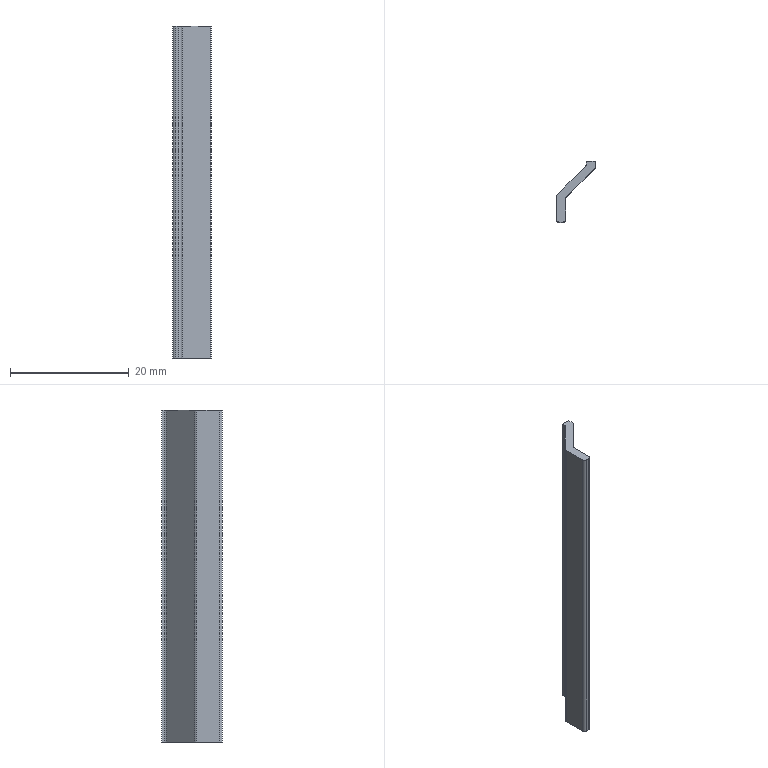Part | NX | features BREP 2 | 2 solids | 32 faces | box 6.515 x 10.276 x 56 mm | volume 1939 mm3 | plane 20 | cylinder 12 | commonest cylinder face diameters 1 x12
STEP:
#1=CARTESIAN_POINT('',(3.258,4.27,-4.));
#2=VERTEX_POINT('',#1);
#3=CARTESIAN_POINT('',(3.258,4.27,52.));
#4=VERTEX_POINT('',#3);
#5=CARTESIAN_POINT('',(3.258,4.27,0.));
#6=DIRECTION('',(0.,0.,1.));
#7=VECTOR('',#6,1000.);
#8=LINE('',#5,#7);
#9=EDGE_CURVE('',#2,#4,#8,.T.);
#10=ORIENTED_EDGE('',*,*,#9,.T.);
#11=CARTESIAN_POINT('',(3.111,3.917,52.));
#12=VERTEX_POINT('',#11);
#13=CARTESIAN_POINT('',(2.758,4.27,52.));
#14=DIRECTION('',(0.,0.,1.));
#15=DIRECTION('',(1.,0.,0.));
#16=AXIS2_PLACEMENT_3D('',#13,#14,#15);
#17=CIRCLE('',#16,0.5);
#18=EDGE_CURVE('',#12,#4,#17,.T.);
#19=ORIENTED_EDGE('',*,*,#18,.F.);
#20=CARTESIAN_POINT('',(3.111,3.917,-4.));
#21=VERTEX_POINT('',#20);
#22=CARTESIAN_POINT('',(3.111,3.917,0.));
#23=DIRECTION('',(0.,0.,1.));
#24=VECTOR('',#23,1000.);
#25=LINE('',#22,#24);
#26=EDGE_CURVE('',#21,#12,#25,.T.);
#27=ORIENTED_EDGE('',*,*,#26,.F.);
#28=CARTESIAN_POINT('',(2.758,4.27,-4.));
#29=DIRECTION('',(0.,0.,1.));
#30=DIRECTION('',(1.,0.,0.));
#31=AXIS2_PLACEMENT_3D('',#28,#29,#30);
#32=CIRCLE('',#31,0.5);
#33=EDGE_CURVE('',#21,#2,#32,.T.);
#34=ORIENTED_EDGE('',*,*,#33,.T.);
#35=EDGE_LOOP('',(#10,#19,#27,#34));
#36=FACE_BOUND('',#35,.T.);
#37=CARTESIAN_POINT('',(2.758,4.27,0.));
#38=DIRECTION('',(0.,0.,1.));
#39=DIRECTION('',(-1.,0.,0.));
#40=AXIS2_PLACEMENT_3D('',#37,#38,#39);
#41=CYLINDRICAL_SURFACE('',#40,0.5);
#42=ADVANCED_FACE('',(#36),#41,.T.);
#43=ORIENTED_EDGE('',*,*,#26,.T.);
#44=CARTESIAN_POINT('',(-1.611,-0.806,52.));
#45=VERTEX_POINT('',#44);
#46=CARTESIAN_POINT('',(3.111,3.917,52.));
#47=DIRECTION('',(0.7071,0.7071,0.));
#48=VECTOR('',#47,1000.);
#49=LINE('',#46,#48);
#50=EDGE_CURVE('',#45,#12,#49,.T.);
#51=ORIENTED_EDGE('',*,*,#50,.F.);
#52=CARTESIAN_POINT('',(-1.611,-0.806,-4.));
#53=VERTEX_POINT('',#52);
#54=CARTESIAN_POINT('',(-1.611,-0.806,0.));
#55=DIRECTION('',(0.,0.,1.));
#56=VECTOR('',#55,1000.);
#57=LINE('',#54,#56);
#58=EDGE_CURVE('',#53,#45,#57,.T.);
#59=ORIENTED_EDGE('',*,*,#58,.F.);
#60=CARTESIAN_POINT('',(3.111,3.917,-4.));
#61=DIRECTION('',(0.7071,0.7071,0.));
#62=VECTOR('',#61,1000.);
#63=LINE('',#60,#62);
#64=EDGE_CURVE('',#53,#21,#63,.T.);
#65=ORIENTED_EDGE('',*,*,#64,.T.);
#66=EDGE_LOOP('',(#43,#51,#59,#65));
#67=FACE_BOUND('',#66,.T.);
#68=CARTESIAN_POINT('',(3.111,3.917,0.));
#69=DIRECTION('',(-0.7071,0.7071,0.));
#70=DIRECTION('',(0.7071,0.7071,0.));
#71=AXIS2_PLACEMENT_3D('',#68,#69,#70);
#72=PLANE('',#71);
#73=ADVANCED_FACE('',(#67),#72,.F.);
#74=ORIENTED_EDGE('',*,*,#58,.T.);
#75=CARTESIAN_POINT('',(-1.758,-1.16,52.));
#76=VERTEX_POINT('',#75);
#77=CARTESIAN_POINT('',(-1.258,-1.16,52.));
#78=DIRECTION('',(0.,0.,-1.));
#79=DIRECTION('',(1.,0.,0.));
#80=AXIS2_PLACEMENT_3D('',#77,#78,#79);
#81=CIRCLE('',#80,0.5);
#82=EDGE_CURVE('',#76,#45,#81,.T.);
#83=ORIENTED_EDGE('',*,*,#82,.F.);
#84=CARTESIAN_POINT('',(-1.758,-1.16,-4.));
#85=VERTEX_POINT('',#84);
#86=CARTESIAN_POINT('',(-1.758,-1.16,0.));
#87=DIRECTION('',(0.,0.,1.));
#88=VECTOR('',#87,1000.);
#89=LINE('',#86,#88);
#90=EDGE_CURVE('',#85,#76,#89,.T.);
#91=ORIENTED_EDGE('',*,*,#90,.F.);
#92=CARTESIAN_POINT('',(-1.258,-1.16,-4.));
#93=DIRECTION('',(0.,0.,-1.));
#94=DIRECTION('',(1.,0.,0.));
#95=AXIS2_PLACEMENT_3D('',#92,#93,#94);
#96=CIRCLE('',#95,0.5);
#97=EDGE_CURVE('',#85,#53,#96,.T.);
#98=ORIENTED_EDGE('',*,*,#97,.T.);
#99=EDGE_LOOP('',(#74,#83,#91,#98));
#100=FACE_BOUND('',#99,.T.);
#101=CARTESIAN_POINT('',(-1.258,-1.16,0.));
#102=DIRECTION('',(0.,0.,1.));
#103=DIRECTION('',(-1.,0.,0.));
#104=AXIS2_PLACEMENT_3D('',#101,#102,#103);
#105=CYLINDRICAL_SURFACE('',#104,0.5);
#106=ADVANCED_FACE('',(#100),#105,.F.);
#107=ORIENTED_EDGE('',*,*,#90,.T.);
#108=CARTESIAN_POINT('',(-1.758,-4.613,52.));
#109=VERTEX_POINT('',#108);
#110=CARTESIAN_POINT('',(-1.758,-7.135,52.));
#111=DIRECTION('',(0.,1.,0.));
#112=VECTOR('',#111,1000.);
#113=LINE('',#110,#112);
#114=EDGE_CURVE('',#109,#76,#113,.T.);
#115=ORIENTED_EDGE('',*,*,#114,.F.);
#116=CARTESIAN_POINT('',(-1.758,-4.613,-4.));
#117=VERTEX_POINT('',#116);
#118=CARTESIAN_POINT('',(-1.758,-4.613,0.));
#119=DIRECTION('',(0.,0.,1.));
#120=VECTOR('',#119,1000.);
#121=LINE('',#118,#120);
#122=EDGE_CURVE('',#117,#109,#121,.T.);
#123=ORIENTED_EDGE('',*,*,#122,.F.);
#124=CARTESIAN_POINT('',(-1.758,-7.135,-4.));
#125=DIRECTION('',(0.,1.,0.));
#126=VECTOR('',#125,1000.);
#127=LINE('',#124,#126);
#128=EDGE_CURVE('',#117,#85,#127,.T.);
#129=ORIENTED_EDGE('',*,*,#128,.T.);
#130=EDGE_LOOP('',(#107,#115,#123,#129));
#131=FACE_BOUND('',#130,.T.);
#132=CARTESIAN_POINT('',(-1.758,-1.16,0.));
#133=DIRECTION('',(-1.,0.,0.));
#134=DIRECTION('',(0.,1.,0.));
#135=AXIS2_PLACEMENT_3D('',#132,#133,#134);
#136=PLANE('',#135);
#137=ADVANCED_FACE('',(#131),#136,.F.);
#138=ORIENTED_EDGE('',*,*,#122,.T.);
#139=CARTESIAN_POINT('',(-2.258,-5.113,52.));
#140=VERTEX_POINT('',#139);
#141=CARTESIAN_POINT('',(-2.258,-4.613,52.));
#142=DIRECTION('',(0.,0.,1.));
#143=DIRECTION('',(1.,0.,0.));
#144=AXIS2_PLACEMENT_3D('',#141,#142,#143);
#145=CIRCLE('',#144,0.5);
#146=EDGE_CURVE('',#140,#109,#145,.T.);
#147=ORIENTED_EDGE('',*,*,#146,.F.);
#148=CARTESIAN_POINT('',(-2.258,-5.113,-4.));
#149=VERTEX_POINT('',#148);
#150=CARTESIAN_POINT('',(-2.258,-5.113,0.));
#151=DIRECTION('',(0.,0.,1.));
#152=VECTOR('',#151,1000.);
#153=LINE('',#150,#152);
#154=EDGE_CURVE('',#149,#140,#153,.T.);
#155=ORIENTED_EDGE('',*,*,#154,.F.);
#156=CARTESIAN_POINT('',(-2.258,-4.613,-4.));
#157=DIRECTION('',(0.,0.,1.));
#158=DIRECTION('',(1.,0.,0.));
#159=AXIS2_PLACEMENT_3D('',#156,#157,#158);
#160=CIRCLE('',#159,0.5);
#161=EDGE_CURVE('',#149,#117,#160,.T.);
#162=ORIENTED_EDGE('',*,*,#161,.T.);
#163=EDGE_LOOP('',(#138,#147,#155,#162));
#164=FACE_BOUND('',#163,.T.);
#165=CARTESIAN_POINT('',(-2.258,-4.613,0.));
#166=DIRECTION('',(0.,0.,1.));
#167=DIRECTION('',(-1.,0.,0.));
#168=AXIS2_PLACEMENT_3D('',#165,#166,#167);
#169=CYLINDRICAL_SURFACE('',#168,0.5);
#170=ADVANCED_FACE('',(#164),#169,.T.);
#171=ORIENTED_EDGE('',*,*,#154,.T.);
#172=CARTESIAN_POINT('',(-2.758,-5.113,52.));
#173=VERTEX_POINT('',#172);
#174=CARTESIAN_POINT('',(2.716,-5.113,52.));
#175=DIRECTION('',(1.,0.,0.));
#176=VECTOR('',#175,1000.);
#177=LINE('',#174,#176);
#178=EDGE_CURVE('',#173,#140,#177,.T.);
#179=ORIENTED_EDGE('',*,*,#178,.F.);
#180=CARTESIAN_POINT('',(-2.758,-5.113,-4.));
#181=VERTEX_POINT('',#180);
#182=CARTESIAN_POINT('',(-2.758,-5.113,0.));
#183=DIRECTION('',(0.,0.,1.));
#184=VECTOR('',#183,1000.);
#185=LINE('',#182,#184);
#186=EDGE_CURVE('',#181,#173,#185,.T.);
#187=ORIENTED_EDGE('',*,*,#186,.F.);
#188=CARTESIAN_POINT('',(2.716,-5.113,-4.));
#189=DIRECTION('',(1.,0.,0.));
#190=VECTOR('',#189,1000.);
#191=LINE('',#188,#190);
#192=EDGE_CURVE('',#181,#149,#191,.T.);
#193=ORIENTED_EDGE('',*,*,#192,.T.);
#194=EDGE_LOOP('',(#171,#179,#187,#193));
#195=FACE_BOUND('',#194,.T.);
#196=CARTESIAN_POINT('',(-2.258,-5.113,0.));
#197=DIRECTION('',(0.,1.,0.));
#198=DIRECTION('',(1.,0.,0.));
#199=AXIS2_PLACEMENT_3D('',#196,#197,#198);
#200=PLANE('',#199);
#201=ADVANCED_FACE('',(#195),#200,.F.);
#202=ORIENTED_EDGE('',*,*,#186,.T.);
#203=CARTESIAN_POINT('',(-3.258,-4.613,52.));
#204=VERTEX_POINT('',#203);
#205=CARTESIAN_POINT('',(-2.758,-4.613,52.));
#206=DIRECTION('',(0.,0.,1.));
#207=DIRECTION('',(1.,0.,0.));
#208=AXIS2_PLACEMENT_3D('',#205,#206,#207);
#209=CIRCLE('',#208,0.5);
#210=EDGE_CURVE('',#204,#173,#209,.T.);
#211=ORIENTED_EDGE('',*,*,#210,.F.);
#212=CARTESIAN_POINT('',(-3.258,-4.613,-4.));
#213=VERTEX_POINT('',#212);
#214=CARTESIAN_POINT('',(-3.258,-4.613,0.));
#215=DIRECTION('',(0.,0.,1.));
#216=VECTOR('',#215,1000.);
#217=LINE('',#214,#216);
#218=EDGE_CURVE('',#213,#204,#217,.T.);
#219=ORIENTED_EDGE('',*,*,#218,.F.);
#220=CARTESIAN_POINT('',(-2.758,-4.613,-4.));
#221=DIRECTION('',(0.,0.,1.));
#222=DIRECTION('',(1.,0.,0.));
#223=AXIS2_PLACEMENT_3D('',#220,#221,#222);
#224=CIRCLE('',#223,0.5);
#225=EDGE_CURVE('',#213,#181,#224,.T.);
#226=ORIENTED_EDGE('',*,*,#225,.T.);
#227=EDGE_LOOP('',(#202,#211,#219,#226));
#228=FACE_BOUND('',#227,.T.);
#229=CARTESIAN_POINT('',(-2.758,-4.613,0.));
#230=DIRECTION('',(0.,0.,1.));
#231=DIRECTION('',(-1.,0.,0.));
#232=AXIS2_PLACEMENT_3D('',#229,#230,#231);
#233=CYLINDRICAL_SURFACE('',#232,0.5);
#234=ADVANCED_FACE('',(#228),#233,.T.);
#235=ORIENTED_EDGE('',*,*,#218,.T.);
#236=CARTESIAN_POINT('',(-3.258,-0.7595,52.));
#237=VERTEX_POINT('',#236);
#238=CARTESIAN_POINT('',(-3.258,-7.135,52.));
#239=DIRECTION('',(0.,-1.,0.));
#240=VECTOR('',#239,1000.);
#241=LINE('',#238,#240);
#242=EDGE_CURVE('',#237,#204,#241,.T.);
#243=ORIENTED_EDGE('',*,*,#242,.F.);
#244=CARTESIAN_POINT('',(-3.258,-0.7595,-4.));
#245=VERTEX_POINT('',#244);
#246=CARTESIAN_POINT('',(-3.258,-0.7595,0.));
#247=DIRECTION('',(0.,0.,1.));
#248=VECTOR('',#247,1000.);
#249=LINE('',#246,#248);
#250=EDGE_CURVE('',#245,#237,#249,.T.);
#251=ORIENTED_EDGE('',*,*,#250,.F.);
#252=CARTESIAN_POINT('',(-3.258,-7.135,-4.));
#253=DIRECTION('',(0.,-1.,0.));
#254=VECTOR('',#253,1000.);
#255=LINE('',#252,#254);
#256=EDGE_CURVE('',#245,#213,#255,.T.);
#257=ORIENTED_EDGE('',*,*,#256,.T.);
#258=EDGE_LOOP('',(#235,#243,#251,#257));
#259=FACE_BOUND('',#258,.T.);
#260=CARTESIAN_POINT('',(-3.258,-4.613,0.));
#261=DIRECTION('',(1.,0.,0.));
#262=DIRECTION('',(0.,-1.,0.));
#263=AXIS2_PLACEMENT_3D('',#260,#261,#262);
#264=PLANE('',#263);
#265=ADVANCED_FACE('',(#259),#264,.F.);
#266=ORIENTED_EDGE('',*,*,#250,.T.);
#267=CARTESIAN_POINT('',(-3.111,-0.406,52.));
#268=VERTEX_POINT('',#267);
#269=CARTESIAN_POINT('',(-2.758,-0.7595,52.));
#270=DIRECTION('',(0.,0.,1.));
#271=DIRECTION('',(1.,0.,0.));
#272=AXIS2_PLACEMENT_3D('',#269,#270,#271);
#273=CIRCLE('',#272,0.5);
#274=EDGE_CURVE('',#268,#237,#273,.T.);
#275=ORIENTED_EDGE('',*,*,#274,.F.);
#276=CARTESIAN_POINT('',(-3.111,-0.406,-4.));
#277=VERTEX_POINT('',#276);
#278=CARTESIAN_POINT('',(-3.111,-0.406,0.));
#279=DIRECTION('',(0.,0.,1.));
#280=VECTOR('',#279,1000.);
#281=LINE('',#278,#280);
#282=EDGE_CURVE('',#277,#268,#281,.T.);
#283=ORIENTED_EDGE('',*,*,#282,.F.);
#284=CARTESIAN_POINT('',(-2.758,-0.7595,-4.));
#285=DIRECTION('',(0.,0.,1.));
#286=DIRECTION('',(1.,0.,0.));
#287=AXIS2_PLACEMENT_3D('',#284,#285,#286);
#288=CIRCLE('',#287,0.5);
#289=EDGE_CURVE('',#277,#245,#288,.T.);
#290=ORIENTED_EDGE('',*,*,#289,.T.);
#291=EDGE_LOOP('',(#266,#275,#283,#290));
#292=FACE_BOUND('',#291,.T.);
#293=CARTESIAN_POINT('',(-2.758,-0.7595,0.));
#294=DIRECTION('',(0.,0.,1.));
#295=DIRECTION('',(-1.,0.,0.));
#296=AXIS2_PLACEMENT_3D('',#293,#294,#295);
#297=CYLINDRICAL_SURFACE('',#296,0.5);
#298=ADVANCED_FACE('',(#292),#297,.T.);
#299=ORIENTED_EDGE('',*,*,#282,.T.);
#300=CARTESIAN_POINT('',(1.611,4.317,52.));
#301=VERTEX_POINT('',#300);
#302=CARTESIAN_POINT('',(-3.111,-0.406,52.));
#303=DIRECTION('',(-0.7071,-0.7071,0.));
#304=VECTOR('',#303,1000.);
#305=LINE('',#302,#304);
#306=EDGE_CURVE('',#301,#268,#305,.T.);
#307=ORIENTED_EDGE('',*,*,#306,.F.);
#308=CARTESIAN_POINT('',(1.611,4.317,-4.));
#309=VERTEX_POINT('',#308);
#310=CARTESIAN_POINT('',(1.611,4.317,0.));
#311=DIRECTION('',(0.,0.,1.));
#312=VECTOR('',#311,1000.);
#313=LINE('',#310,#312);
#314=EDGE_CURVE('',#309,#301,#313,.T.);
#315=ORIENTED_EDGE('',*,*,#314,.F.);
#316=CARTESIAN_POINT('',(-3.111,-0.406,-4.));
#317=DIRECTION('',(-0.7071,-0.7071,0.));
#318=VECTOR('',#317,1000.);
#319=LINE('',#316,#318);
#320=EDGE_CURVE('',#309,#277,#319,.T.);
#321=ORIENTED_EDGE('',*,*,#320,.T.);
#322=EDGE_LOOP('',(#299,#307,#315,#321));
#323=FACE_BOUND('',#322,.T.);
#324=CARTESIAN_POINT('',(-3.111,-0.406,0.));
#325=DIRECTION('',(0.7071,-0.7071,0.));
#326=DIRECTION('',(-0.7071,-0.7071,0.));
#327=AXIS2_PLACEMENT_3D('',#324,#325,#326);
#328=PLANE('',#327);
#329=ADVANCED_FACE('',(#323),#328,.F.);
#330=ORIENTED_EDGE('',*,*,#314,.T.);
#331=CARTESIAN_POINT('',(1.758,4.67,52.));
#332=VERTEX_POINT('',#331);
#333=CARTESIAN_POINT('',(1.258,4.67,52.));
#334=DIRECTION('',(0.,0.,-1.));
#335=DIRECTION('',(1.,0.,0.));
#336=AXIS2_PLACEMENT_3D('',#333,#334,#335);
#337=CIRCLE('',#336,0.5);
#338=EDGE_CURVE('',#332,#301,#337,.T.);
#339=ORIENTED_EDGE('',*,*,#338,.F.);
#340=CARTESIAN_POINT('',(1.758,4.67,-4.));
#341=VERTEX_POINT('',#340);
#342=CARTESIAN_POINT('',(1.758,4.67,0.));
#343=DIRECTION('',(0.,0.,1.));
#344=VECTOR('',#343,1000.);
#345=LINE('',#342,#344);
#346=EDGE_CURVE('',#341,#332,#345,.T.);
#347=ORIENTED_EDGE('',*,*,#346,.F.);
#348=CARTESIAN_POINT('',(1.258,4.67,-4.));
#349=DIRECTION('',(0.,0.,-1.));
#350=DIRECTION('',(1.,0.,0.));
#351=AXIS2_PLACEMENT_3D('',#348,#349,#350);
#352=CIRCLE('',#351,0.5);
#353=EDGE_CURVE('',#341,#309,#352,.T.);
#354=ORIENTED_EDGE('',*,*,#353,.T.);
#355=EDGE_LOOP('',(#330,#339,#347,#354));
#356=FACE_BOUND('',#355,.T.);
#357=CARTESIAN_POINT('',(1.258,4.67,0.));
#358=DIRECTION('',(0.,0.,1.));
#359=DIRECTION('',(-1.,0.,0.));
#360=AXIS2_PLACEMENT_3D('',#357,#358,#359);
#361=CYLINDRICAL_SURFACE('',#360,0.5);
#362=ADVANCED_FACE('',(#356),#361,.F.);
#363=ORIENTED_EDGE('',*,*,#346,.T.);
#364=CARTESIAN_POINT('',(1.758,5.163,52.));
#365=VERTEX_POINT('',#364);
#366=CARTESIAN_POINT('',(1.758,-7.135,52.));
#367=DIRECTION('',(0.,-1.,0.));
#368=VECTOR('',#367,1000.);
#369=LINE('',#366,#368);
#370=EDGE_CURVE('',#365,#332,#369,.T.);
#371=ORIENTED_EDGE('',*,*,#370,.F.);
#372=CARTESIAN_POINT('',(1.758,5.163,-4.));
#373=VERTEX_POINT('',#372);
#374=CARTESIAN_POINT('',(1.758,5.163,0.));
#375=DIRECTION('',(0.,0.,1.));
#376=VECTOR('',#375,1000.);
#377=LINE('',#374,#376);
#378=EDGE_CURVE('',#373,#365,#377,.T.);
#379=ORIENTED_EDGE('',*,*,#378,.F.);
#380=CARTESIAN_POINT('',(1.758,-7.135,-4.));
#381=DIRECTION('',(0.,-1.,0.));
#382=VECTOR('',#381,1000.);
#383=LINE('',#380,#382);
#384=EDGE_CURVE('',#373,#341,#383,.T.);
#385=ORIENTED_EDGE('',*,*,#384,.T.);
#386=EDGE_LOOP('',(#363,#371,#379,#385));
#387=FACE_BOUND('',#386,.T.);
#388=CARTESIAN_POINT('',(1.758,4.67,0.));
#389=DIRECTION('',(1.,0.,0.));
#390=DIRECTION('',(0.,-1.,0.));
#391=AXIS2_PLACEMENT_3D('',#388,#389,#390);
#392=PLANE('',#391);
#393=ADVANCED_FACE('',(#387),#392,.F.);
#394=ORIENTED_EDGE('',*,*,#378,.T.);
#395=CARTESIAN_POINT('',(3.258,5.163,52.));
#396=VERTEX_POINT('',#395);
#397=CARTESIAN_POINT('',(2.716,5.163,52.));
#398=DIRECTION('',(-1.,0.,0.));
#399=VECTOR('',#398,1000.);
#400=LINE('',#397,#399);
#401=EDGE_CURVE('',#396,#365,#400,.T.);
#402=ORIENTED_EDGE('',*,*,#401,.F.);
#403=CARTESIAN_POINT('',(3.258,5.163,-4.));
#404=VERTEX_POINT('',#403);
#405=CARTESIAN_POINT('',(3.258,5.163,0.));
#406=DIRECTION('',(0.,0.,1.));
#407=VECTOR('',#406,1000.);
#408=LINE('',#405,#407);
#409=EDGE_CURVE('',#404,#396,#408,.T.);
#410=ORIENTED_EDGE('',*,*,#409,.F.);
#411=CARTESIAN_POINT('',(2.716,5.163,-4.));
#412=DIRECTION('',(-1.,0.,0.));
#413=VECTOR('',#412,1000.);
#414=LINE('',#411,#413);
#415=EDGE_CURVE('',#404,#373,#414,.T.);
#416=ORIENTED_EDGE('',*,*,#415,.T.);
#417=EDGE_LOOP('',(#394,#402,#410,#416));
#418=FACE_BOUND('',#417,.T.);
#419=CARTESIAN_POINT('',(2.716,5.163,0.));
#420=DIRECTION('',(0.,-1.,0.));
#421=DIRECTION('',(-1.,0.,0.));
#422=AXIS2_PLACEMENT_3D('',#419,#420,#421);
#423=PLANE('',#422);
#424=ADVANCED_FACE('',(#418),#423,.F.);
#425=CARTESIAN_POINT('',(3.258,-7.135,-4.));
#426=DIRECTION('',(0.,1.,0.));
#427=VECTOR('',#426,1000.);
#428=LINE('',#425,#427);
#429=EDGE_CURVE('',#2,#404,#428,.T.);
#430=ORIENTED_EDGE('',*,*,#429,.T.);
#431=ORIENTED_EDGE('',*,*,#409,.T.);
#432=CARTESIAN_POINT('',(3.258,-7.135,52.));
#433=DIRECTION('',(0.,1.,0.));
#434=VECTOR('',#433,1000.);
#435=LINE('',#432,#434);
#436=EDGE_CURVE('',#4,#396,#435,.T.);
#437=ORIENTED_EDGE('',*,*,#436,.F.);
#438=ORIENTED_EDGE('',*,*,#9,.F.);
#439=EDGE_LOOP('',(#430,#431,#437,#438));
#440=FACE_BOUND('',#439,.T.);
#441=CARTESIAN_POINT('',(3.258,10.163,0.));
#442=DIRECTION('',(-1.,0.,0.));
#443=DIRECTION('',(0.,1.,0.));
#444=AXIS2_PLACEMENT_3D('',#441,#442,#443);
#445=PLANE('',#444);
#446=ADVANCED_FACE('',(#440),#445,.F.);
#447=ORIENTED_EDGE('',*,*,#401,.T.);
#448=ORIENTED_EDGE('',*,*,#370,.T.);
#449=ORIENTED_EDGE('',*,*,#338,.T.);
#450=ORIENTED_EDGE('',*,*,#306,.T.);
#451=ORIENTED_EDGE('',*,*,#274,.T.);
#452=ORIENTED_EDGE('',*,*,#242,.T.);
#453=ORIENTED_EDGE('',*,*,#210,.T.);
#454=ORIENTED_EDGE('',*,*,#178,.T.);
#455=ORIENTED_EDGE('',*,*,#146,.T.);
#456=ORIENTED_EDGE('',*,*,#114,.T.);
#457=ORIENTED_EDGE('',*,*,#82,.T.);
#458=ORIENTED_EDGE('',*,*,#50,.T.);
#459=ORIENTED_EDGE('',*,*,#18,.T.);
#460=ORIENTED_EDGE('',*,*,#436,.T.);
#461=EDGE_LOOP('',(#447,#448,#449,#450,#451,#452,#453,#454,#455,#456,#457,#458,#459,#460));
#462=FACE_BOUND('',#461,.T.);
#463=CARTESIAN_POINT('',(2.716,-7.135,52.));
#464=DIRECTION('',(0.,0.,1.));
#465=DIRECTION('',(-1.,0.,0.));
#466=AXIS2_PLACEMENT_3D('',#463,#464,#465);
#467=PLANE('',#466);
#468=ADVANCED_FACE('',(#462),#467,.T.);
#469=ORIENTED_EDGE('',*,*,#415,.F.);
#470=ORIENTED_EDGE('',*,*,#429,.F.);
#471=ORIENTED_EDGE('',*,*,#33,.F.);
#472=ORIENTED_EDGE('',*,*,#64,.F.);
#473=ORIENTED_EDGE('',*,*,#97,.F.);
#474=ORIENTED_EDGE('',*,*,#128,.F.);
#475=ORIENTED_EDGE('',*,*,#161,.F.);
#476=ORIENTED_EDGE('',*,*,#192,.F.);
#477=ORIENTED_EDGE('',*,*,#225,.F.);
#478=ORIENTED_EDGE('',*,*,#256,.F.);
#479=ORIENTED_EDGE('',*,*,#289,.F.);
#480=ORIENTED_EDGE('',*,*,#320,.F.);
#481=ORIENTED_EDGE('',*,*,#353,.F.);
#482=ORIENTED_EDGE('',*,*,#384,.F.);
#483=EDGE_LOOP('',(#469,#470,#471,#472,#473,#474,#475,#476,#477,#478,#479,#480,#481,#482));
#484=FACE_BOUND('',#483,.T.);
#485=CARTESIAN_POINT('',(2.716,-7.135,-4.));
#486=DIRECTION('',(0.,0.,1.));
#487=DIRECTION('',(-1.,0.,0.));
#488=AXIS2_PLACEMENT_3D('',#485,#486,#487);
#489=PLANE('',#488);
#490=ADVANCED_FACE('',(#484),#489,.F.);
#491=CLOSED_SHELL('',(#42,#73,#106,#137,#170,#201,#234,#265,#298,#329,#362,#393,#424,#446,#468,#490));
#492=MANIFOLD_SOLID_BREP('',#491);
#493=CARTESIAN_POINT('',(3.258,4.27,-4.));
#494=VERTEX_POINT('',#493);
#495=CARTESIAN_POINT('',(3.258,4.27,52.));
#496=VERTEX_POINT('',#495);
#497=CARTESIAN_POINT('',(3.258,4.27,0.));
#498=DIRECTION('',(0.,0.,1.));
#499=VECTOR('',#498,1000.);
#500=LINE('',#497,#499);
#501=EDGE_CURVE('',#494,#496,#500,.T.);
#502=ORIENTED_EDGE('',*,*,#501,.T.);
#503=CARTESIAN_POINT('',(3.111,3.917,52.));
#504=VERTEX_POINT('',#503);
#505=CARTESIAN_POINT('',(2.758,4.27,52.));
#506=DIRECTION('',(0.,0.,1.));
#507=DIRECTION('',(1.,0.,0.));
#508=AXIS2_PLACEMENT_3D('',#505,#506,#507);
#509=CIRCLE('',#508,0.5);
#510=EDGE_CURVE('',#504,#496,#509,.T.);
#511=ORIENTED_EDGE('',*,*,#510,.F.);
#512=CARTESIAN_POINT('',(3.111,3.917,-4.));
#513=VERTEX_POINT('',#512);
#514=CARTESIAN_POINT('',(3.111,3.917,0.));
#515=DIRECTION('',(0.,0.,1.));
#516=VECTOR('',#515,1000.);
#517=LINE('',#514,#516);
#518=EDGE_CURVE('',#513,#504,#517,.T.);
#519=ORIENTED_EDGE('',*,*,#518,.F.);
#520=CARTESIAN_POINT('',(2.758,4.27,-4.));
#521=DIRECTION('',(0.,0.,1.));
#522=DIRECTION('',(1.,0.,0.));
#523=AXIS2_PLACEMENT_3D('',#520,#521,#522);
#524=CIRCLE('',#523,0.5);
#525=EDGE_CURVE('',#513,#494,#524,.T.);
#526=ORIENTED_EDGE('',*,*,#525,.T.);
#527=EDGE_LOOP('',(#502,#511,#519,#526));
#528=FACE_BOUND('',#527,.T.);
#529=CARTESIAN_POINT('',(2.758,4.27,0.));
#530=DIRECTION('',(0.,0.,1.));
#531=DIRECTION('',(-1.,0.,0.));
#532=AXIS2_PLACEMENT_3D('',#529,#530,#531);
#533=CYLINDRICAL_SURFACE('',#532,0.5);
#534=ADVANCED_FACE('',(#528),#533,.T.);
#535=ORIENTED_EDGE('',*,*,#518,.T.);
#536=CARTESIAN_POINT('',(-1.611,-0.806,52.));
#537=VERTEX_POINT('',#536);
#538=CARTESIAN_POINT('',(3.111,3.917,52.));
#539=DIRECTION('',(0.7071,0.7071,0.));
#540=VECTOR('',#539,1000.);
#541=LINE('',#538,#540);
#542=EDGE_CURVE('',#537,#504,#541,.T.);
#543=ORIENTED_EDGE('',*,*,#542,.F.);
#544=CARTESIAN_POINT('',(-1.611,-0.806,-4.));
#545=VERTEX_POINT('',#544);
#546=CARTESIAN_POINT('',(-1.611,-0.806,0.));
#547=DIRECTION('',(0.,0.,1.));
#548=VECTOR('',#547,1000.);
#549=LINE('',#546,#548);
#550=EDGE_CURVE('',#545,#537,#549,.T.);
#551=ORIENTED_EDGE('',*,*,#550,.F.);
#552=CARTESIAN_POINT('',(3.111,3.917,-4.));
#553=DIRECTION('',(0.7071,0.7071,0.));
#554=VECTOR('',#553,1000.);
#555=LINE('',#552,#554);
#556=EDGE_CURVE('',#545,#513,#555,.T.);
#557=ORIENTED_EDGE('',*,*,#556,.T.);
#558=EDGE_LOOP('',(#535,#543,#551,#557));
#559=FACE_BOUND('',#558,.T.);
#560=CARTESIAN_POINT('',(3.111,3.917,0.));
#561=DIRECTION('',(-0.7071,0.7071,0.));
#562=DIRECTION('',(0.7071,0.7071,0.));
#563=AXIS2_PLACEMENT_3D('',#560,#561,#562);
#564=PLANE('',#563);
#565=ADVANCED_FACE('',(#559),#564,.F.);
#566=ORIENTED_EDGE('',*,*,#550,.T.);
#567=CARTESIAN_POINT('',(-1.758,-1.16,52.));
#568=VERTEX_POINT('',#567);
#569=CARTESIAN_POINT('',(-1.258,-1.16,52.));
#570=DIRECTION('',(0.,0.,-1.));
#571=DIRECTION('',(1.,0.,0.));
#572=AXIS2_PLACEMENT_3D('',#569,#570,#571);
#573=CIRCLE('',#572,0.5);
#574=EDGE_CURVE('',#568,#537,#573,.T.);
#575=ORIENTED_EDGE('',*,*,#574,.F.);
#576=CARTESIAN_POINT('',(-1.758,-1.16,-4.));
#577=VERTEX_POINT('',#576);
#578=CARTESIAN_POINT('',(-1.758,-1.16,0.));
#579=DIRECTION('',(0.,0.,1.));
#580=VECTOR('',#579,1000.);
#581=LINE('',#578,#580);
#582=EDGE_CURVE('',#577,#568,#581,.T.);
#583=ORIENTED_EDGE('',*,*,#582,.F.);
#584=CARTESIAN_POINT('',(-1.258,-1.16,-4.));
#585=DIRECTION('',(0.,0.,-1.));
#586=DIRECTION('',(1.,0.,0.));
#587=AXIS2_PLACEMENT_3D('',#584,#585,#586);
#588=CIRCLE('',#587,0.5);
#589=EDGE_CURVE('',#577,#545,#588,.T.);
#590=ORIENTED_EDGE('',*,*,#589,.T.);
#591=EDGE_LOOP('',(#566,#575,#583,#590));
#592=FACE_BOUND('',#591,.T.);
#593=CARTESIAN_POINT('',(-1.258,-1.16,0.));
#594=DIRECTION('',(0.,0.,1.));
#595=DIRECTION('',(-1.,0.,0.));
#596=AXIS2_PLACEMENT_3D('',#593,#594,#595);
#597=CYLINDRICAL_SURFACE('',#596,0.5);
#598=ADVANCED_FACE('',(#592),#597,.F.);
#599=ORIENTED_EDGE('',*,*,#582,.T.);
#600=CARTESIAN_POINT('',(-1.758,-4.613,52.));
#601=VERTEX_POINT('',#600);
#602=CARTESIAN_POINT('',(-1.758,-7.135,52.));
#603=DIRECTION('',(0.,1.,0.));
#604=VECTOR('',#603,1000.);
#605=LINE('',#602,#604);
#606=EDGE_CURVE('',#601,#568,#605,.T.);
#607=ORIENTED_EDGE('',*,*,#606,.F.);
#608=CARTESIAN_POINT('',(-1.758,-4.613,-4.));
#609=VERTEX_POINT('',#608);
#610=CARTESIAN_POINT('',(-1.758,-4.613,0.));
#611=DIRECTION('',(0.,0.,1.));
#612=VECTOR('',#611,1000.);
#613=LINE('',#610,#612);
#614=EDGE_CURVE('',#609,#601,#613,.T.);
#615=ORIENTED_EDGE('',*,*,#614,.F.);
#616=CARTESIAN_POINT('',(-1.758,-7.135,-4.));
#617=DIRECTION('',(0.,1.,0.));
#618=VECTOR('',#617,1000.);
#619=LINE('',#616,#618);
#620=EDGE_CURVE('',#609,#577,#619,.T.);
#621=ORIENTED_EDGE('',*,*,#620,.T.);
#622=EDGE_LOOP('',(#599,#607,#615,#621));
#623=FACE_BOUND('',#622,.T.);
#624=CARTESIAN_POINT('',(-1.758,-1.16,0.));
#625=DIRECTION('',(-1.,0.,0.));
#626=DIRECTION('',(0.,1.,0.));
#627=AXIS2_PLACEMENT_3D('',#624,#625,#626);
#628=PLANE('',#627);
#629=ADVANCED_FACE('',(#623),#628,.F.);
#630=ORIENTED_EDGE('',*,*,#614,.T.);
#631=CARTESIAN_POINT('',(-2.258,-5.113,52.));
#632=VERTEX_POINT('',#631);
#633=CARTESIAN_POINT('',(-2.258,-4.613,52.));
#634=DIRECTION('',(0.,0.,1.));
#635=DIRECTION('',(1.,0.,0.));
#636=AXIS2_PLACEMENT_3D('',#633,#634,#635);
#637=CIRCLE('',#636,0.5);
#638=EDGE_CURVE('',#632,#601,#637,.T.);
#639=ORIENTED_EDGE('',*,*,#638,.F.);
#640=CARTESIAN_POINT('',(-2.258,-5.113,-4.));
#641=VERTEX_POINT('',#640);
#642=CARTESIAN_POINT('',(-2.258,-5.113,0.));
#643=DIRECTION('',(0.,0.,1.));
#644=VECTOR('',#643,1000.);
#645=LINE('',#642,#644);
#646=EDGE_CURVE('',#641,#632,#645,.T.);
#647=ORIENTED_EDGE('',*,*,#646,.F.);
#648=CARTESIAN_POINT('',(-2.258,-4.613,-4.));
#649=DIRECTION('',(0.,0.,1.));
#650=DIRECTION('',(1.,0.,0.));
#651=AXIS2_PLACEMENT_3D('',#648,#649,#650);
#652=CIRCLE('',#651,0.5);
#653=EDGE_CURVE('',#641,#609,#652,.T.);
#654=ORIENTED_EDGE('',*,*,#653,.T.);
#655=EDGE_LOOP('',(#630,#639,#647,#654));
#656=FACE_BOUND('',#655,.T.);
#657=CARTESIAN_POINT('',(-2.258,-4.613,0.));
#658=DIRECTION('',(0.,0.,1.));
#659=DIRECTION('',(-1.,0.,0.));
#660=AXIS2_PLACEMENT_3D('',#657,#658,#659);
#661=CYLINDRICAL_SURFACE('',#660,0.5);
#662=ADVANCED_FACE('',(#656),#661,.T.);
#663=ORIENTED_EDGE('',*,*,#646,.T.);
#664=CARTESIAN_POINT('',(-2.758,-5.113,52.));
#665=VERTEX_POINT('',#664);
#666=CARTESIAN_POINT('',(2.716,-5.113,52.));
#667=DIRECTION('',(1.,0.,0.));
#668=VECTOR('',#667,1000.);
#669=LINE('',#666,#668);
#670=EDGE_CURVE('',#665,#632,#669,.T.);
#671=ORIENTED_EDGE('',*,*,#670,.F.);
#672=CARTESIAN_POINT('',(-2.758,-5.113,-4.));
#673=VERTEX_POINT('',#672);
#674=CARTESIAN_POINT('',(-2.758,-5.113,0.));
#675=DIRECTION('',(0.,0.,1.));
#676=VECTOR('',#675,1000.);
#677=LINE('',#674,#676);
#678=EDGE_CURVE('',#673,#665,#677,.T.);
#679=ORIENTED_EDGE('',*,*,#678,.F.);
#680=CARTESIAN_POINT('',(2.716,-5.113,-4.));
#681=DIRECTION('',(1.,0.,0.));
#682=VECTOR('',#681,1000.);
#683=LINE('',#680,#682);
#684=EDGE_CURVE('',#673,#641,#683,.T.);
#685=ORIENTED_EDGE('',*,*,#684,.T.);
#686=EDGE_LOOP('',(#663,#671,#679,#685));
#687=FACE_BOUND('',#686,.T.);
#688=CARTESIAN_POINT('',(-2.258,-5.113,0.));
#689=DIRECTION('',(0.,1.,0.));
#690=DIRECTION('',(1.,0.,0.));
#691=AXIS2_PLACEMENT_3D('',#688,#689,#690);
#692=PLANE('',#691);
#693=ADVANCED_FACE('',(#687),#692,.F.);
#694=ORIENTED_EDGE('',*,*,#678,.T.);
#695=CARTESIAN_POINT('',(-3.258,-4.613,52.));
#696=VERTEX_POINT('',#695);
#697=CARTESIAN_POINT('',(-2.758,-4.613,52.));
#698=DIRECTION('',(0.,0.,1.));
#699=DIRECTION('',(1.,0.,0.));
#700=AXIS2_PLACEMENT_3D('',#697,#698,#699);
#701=CIRCLE('',#700,0.5);
#702=EDGE_CURVE('',#696,#665,#701,.T.);
#703=ORIENTED_EDGE('',*,*,#702,.F.);
#704=CARTESIAN_POINT('',(-3.258,-4.613,-4.));
#705=VERTEX_POINT('',#704);
#706=CARTESIAN_POINT('',(-3.258,-4.613,0.));
#707=DIRECTION('',(0.,0.,1.));
#708=VECTOR('',#707,1000.);
#709=LINE('',#706,#708);
#710=EDGE_CURVE('',#705,#696,#709,.T.);
#711=ORIENTED_EDGE('',*,*,#710,.F.);
#712=CARTESIAN_POINT('',(-2.758,-4.613,-4.));
#713=DIRECTION('',(0.,0.,1.));
#714=DIRECTION('',(1.,0.,0.));
#715=AXIS2_PLACEMENT_3D('',#712,#713,#714);
#716=CIRCLE('',#715,0.5);
#717=EDGE_CURVE('',#705,#673,#716,.T.);
#718=ORIENTED_EDGE('',*,*,#717,.T.);
#719=EDGE_LOOP('',(#694,#703,#711,#718));
#720=FACE_BOUND('',#719,.T.);
#721=CARTESIAN_POINT('',(-2.758,-4.613,0.));
#722=DIRECTION('',(0.,0.,1.));
#723=DIRECTION('',(-1.,0.,0.));
#724=AXIS2_PLACEMENT_3D('',#721,#722,#723);
#725=CYLINDRICAL_SURFACE('',#724,0.5);
#726=ADVANCED_FACE('',(#720),#725,.T.);
#727=ORIENTED_EDGE('',*,*,#710,.T.);
#728=CARTESIAN_POINT('',(-3.258,-0.7595,52.));
#729=VERTEX_POINT('',#728);
#730=CARTESIAN_POINT('',(-3.258,-7.135,52.));
#731=DIRECTION('',(0.,-1.,0.));
#732=VECTOR('',#731,1000.);
#733=LINE('',#730,#732);
#734=EDGE_CURVE('',#729,#696,#733,.T.);
#735=ORIENTED_EDGE('',*,*,#734,.F.);
#736=CARTESIAN_POINT('',(-3.258,-0.7595,-4.));
#737=VERTEX_POINT('',#736);
#738=CARTESIAN_POINT('',(-3.258,-0.7595,0.));
#739=DIRECTION('',(0.,0.,1.));
#740=VECTOR('',#739,1000.);
#741=LINE('',#738,#740);
#742=EDGE_CURVE('',#737,#729,#741,.T.);
#743=ORIENTED_EDGE('',*,*,#742,.F.);
#744=CARTESIAN_POINT('',(-3.258,-7.135,-4.));
#745=DIRECTION('',(0.,-1.,0.));
#746=VECTOR('',#745,1000.);
#747=LINE('',#744,#746);
#748=EDGE_CURVE('',#737,#705,#747,.T.);
#749=ORIENTED_EDGE('',*,*,#748,.T.);
#750=EDGE_LOOP('',(#727,#735,#743,#749));
#751=FACE_BOUND('',#750,.T.);
#752=CARTESIAN_POINT('',(-3.258,-4.613,0.));
#753=DIRECTION('',(1.,0.,0.));
#754=DIRECTION('',(0.,-1.,0.));
#755=AXIS2_PLACEMENT_3D('',#752,#753,#754);
#756=PLANE('',#755);
#757=ADVANCED_FACE('',(#751),#756,.F.);
#758=ORIENTED_EDGE('',*,*,#742,.T.);
#759=CARTESIAN_POINT('',(-3.111,-0.406,52.));
#760=VERTEX_POINT('',#759);
#761=CARTESIAN_POINT('',(-2.758,-0.7595,52.));
#762=DIRECTION('',(0.,0.,1.));
#763=DIRECTION('',(1.,0.,0.));
#764=AXIS2_PLACEMENT_3D('',#761,#762,#763);
#765=CIRCLE('',#764,0.5);
#766=EDGE_CURVE('',#760,#729,#765,.T.);
#767=ORIENTED_EDGE('',*,*,#766,.F.);
#768=CARTESIAN_POINT('',(-3.111,-0.406,-4.));
#769=VERTEX_POINT('',#768);
#770=CARTESIAN_POINT('',(-3.111,-0.406,0.));
#771=DIRECTION('',(0.,0.,1.));
#772=VECTOR('',#771,1000.);
#773=LINE('',#770,#772);
#774=EDGE_CURVE('',#769,#760,#773,.T.);
#775=ORIENTED_EDGE('',*,*,#774,.F.);
#776=CARTESIAN_POINT('',(-2.758,-0.7595,-4.));
#777=DIRECTION('',(0.,0.,1.));
#778=DIRECTION('',(1.,0.,0.));
#779=AXIS2_PLACEMENT_3D('',#776,#777,#778);
#780=CIRCLE('',#779,0.5);
#781=EDGE_CURVE('',#769,#737,#780,.T.);
#782=ORIENTED_EDGE('',*,*,#781,.T.);
#783=EDGE_LOOP('',(#758,#767,#775,#782));
#784=FACE_BOUND('',#783,.T.);
#785=CARTESIAN_POINT('',(-2.758,-0.7595,0.));
#786=DIRECTION('',(0.,0.,1.));
#787=DIRECTION('',(-1.,0.,0.));
#788=AXIS2_PLACEMENT_3D('',#785,#786,#787);
#789=CYLINDRICAL_SURFACE('',#788,0.5);
#790=ADVANCED_FACE('',(#784),#789,.T.);
#791=ORIENTED_EDGE('',*,*,#774,.T.);
#792=CARTESIAN_POINT('',(1.611,4.317,52.));
#793=VERTEX_POINT('',#792);
#794=CARTESIAN_POINT('',(-3.111,-0.406,52.));
#795=DIRECTION('',(-0.7071,-0.7071,0.));
#796=VECTOR('',#795,1000.);
#797=LINE('',#794,#796);
#798=EDGE_CURVE('',#793,#760,#797,.T.);
#799=ORIENTED_EDGE('',*,*,#798,.F.);
#800=CARTESIAN_POINT('',(1.611,4.317,-4.));
#801=VERTEX_POINT('',#800);
#802=CARTESIAN_POINT('',(1.611,4.317,0.));
#803=DIRECTION('',(0.,0.,1.));
#804=VECTOR('',#803,1000.);
#805=LINE('',#802,#804);
#806=EDGE_CURVE('',#801,#793,#805,.T.);
#807=ORIENTED_EDGE('',*,*,#806,.F.);
#808=CARTESIAN_POINT('',(-3.111,-0.406,-4.));
#809=DIRECTION('',(-0.7071,-0.7071,0.));
#810=VECTOR('',#809,1000.);
#811=LINE('',#808,#810);
#812=EDGE_CURVE('',#801,#769,#811,.T.);
#813=ORIENTED_EDGE('',*,*,#812,.T.);
#814=EDGE_LOOP('',(#791,#799,#807,#813));
#815=FACE_BOUND('',#814,.T.);
#816=CARTESIAN_POINT('',(-3.111,-0.406,0.));
#817=DIRECTION('',(0.7071,-0.7071,0.));
#818=DIRECTION('',(-0.7071,-0.7071,0.));
#819=AXIS2_PLACEMENT_3D('',#816,#817,#818);
#820=PLANE('',#819);
#821=ADVANCED_FACE('',(#815),#820,.F.);
#822=ORIENTED_EDGE('',*,*,#806,.T.);
#823=CARTESIAN_POINT('',(1.758,4.67,52.));
#824=VERTEX_POINT('',#823);
#825=CARTESIAN_POINT('',(1.258,4.67,52.));
#826=DIRECTION('',(0.,0.,-1.));
#827=DIRECTION('',(1.,0.,0.));
#828=AXIS2_PLACEMENT_3D('',#825,#826,#827);
#829=CIRCLE('',#828,0.5);
#830=EDGE_CURVE('',#824,#793,#829,.T.);
#831=ORIENTED_EDGE('',*,*,#830,.F.);
#832=CARTESIAN_POINT('',(1.758,4.67,-4.));
#833=VERTEX_POINT('',#832);
#834=CARTESIAN_POINT('',(1.758,4.67,0.));
#835=DIRECTION('',(0.,0.,1.));
#836=VECTOR('',#835,1000.);
#837=LINE('',#834,#836);
#838=EDGE_CURVE('',#833,#824,#837,.T.);
#839=ORIENTED_EDGE('',*,*,#838,.F.);
#840=CARTESIAN_POINT('',(1.258,4.67,-4.));
#841=DIRECTION('',(0.,0.,-1.));
#842=DIRECTION('',(1.,0.,0.));
#843=AXIS2_PLACEMENT_3D('',#840,#841,#842);
#844=CIRCLE('',#843,0.5);
#845=EDGE_CURVE('',#833,#801,#844,.T.);
#846=ORIENTED_EDGE('',*,*,#845,.T.);
#847=EDGE_LOOP('',(#822,#831,#839,#846));
#848=FACE_BOUND('',#847,.T.);
#849=CARTESIAN_POINT('',(1.258,4.67,0.));
#850=DIRECTION('',(0.,0.,1.));
#851=DIRECTION('',(-1.,0.,0.));
#852=AXIS2_PLACEMENT_3D('',#849,#850,#851);
#853=CYLINDRICAL_SURFACE('',#852,0.5);
#854=ADVANCED_FACE('',(#848),#853,.F.);
#855=ORIENTED_EDGE('',*,*,#838,.T.);
#856=CARTESIAN_POINT('',(1.758,5.163,52.));
#857=VERTEX_POINT('',#856);
#858=CARTESIAN_POINT('',(1.758,-7.135,52.));
#859=DIRECTION('',(0.,-1.,0.));
#860=VECTOR('',#859,1000.);
#861=LINE('',#858,#860);
#862=EDGE_CURVE('',#857,#824,#861,.T.);
#863=ORIENTED_EDGE('',*,*,#862,.F.);
#864=CARTESIAN_POINT('',(1.758,5.163,-4.));
#865=VERTEX_POINT('',#864);
#866=CARTESIAN_POINT('',(1.758,5.163,0.));
#867=DIRECTION('',(0.,0.,1.));
#868=VECTOR('',#867,1000.);
#869=LINE('',#866,#868);
#870=EDGE_CURVE('',#865,#857,#869,.T.);
#871=ORIENTED_EDGE('',*,*,#870,.F.);
#872=CARTESIAN_POINT('',(1.758,-7.135,-4.));
#873=DIRECTION('',(0.,-1.,0.));
#874=VECTOR('',#873,1000.);
#875=LINE('',#872,#874);
#876=EDGE_CURVE('',#865,#833,#875,.T.);
#877=ORIENTED_EDGE('',*,*,#876,.T.);
#878=EDGE_LOOP('',(#855,#863,#871,#877));
#879=FACE_BOUND('',#878,.T.);
#880=CARTESIAN_POINT('',(1.758,4.67,0.));
#881=DIRECTION('',(1.,0.,0.));
#882=DIRECTION('',(0.,-1.,0.));
#883=AXIS2_PLACEMENT_3D('',#880,#881,#882);
#884=PLANE('',#883);
#885=ADVANCED_FACE('',(#879),#884,.F.);
#886=ORIENTED_EDGE('',*,*,#870,.T.);
#887=CARTESIAN_POINT('',(3.258,5.163,52.));
#888=VERTEX_POINT('',#887);
#889=CARTESIAN_POINT('',(2.716,5.163,52.));
#890=DIRECTION('',(-1.,0.,0.));
#891=VECTOR('',#890,1000.);
#892=LINE('',#889,#891);
#893=EDGE_CURVE('',#888,#857,#892,.T.);
#894=ORIENTED_EDGE('',*,*,#893,.F.);
#895=CARTESIAN_POINT('',(3.258,5.163,-4.));
#896=VERTEX_POINT('',#895);
#897=CARTESIAN_POINT('',(3.258,5.163,0.));
#898=DIRECTION('',(0.,0.,1.));
#899=VECTOR('',#898,1000.);
#900=LINE('',#897,#899);
#901=EDGE_CURVE('',#896,#888,#900,.T.);
#902=ORIENTED_EDGE('',*,*,#901,.F.);
#903=CARTESIAN_POINT('',(2.716,5.163,-4.));
#904=DIRECTION('',(-1.,0.,0.));
#905=VECTOR('',#904,1000.);
#906=LINE('',#903,#905);
#907=EDGE_CURVE('',#896,#865,#906,.T.);
#908=ORIENTED_EDGE('',*,*,#907,.T.);
#909=EDGE_LOOP('',(#886,#894,#902,#908));
#910=FACE_BOUND('',#909,.T.);
#911=CARTESIAN_POINT('',(2.716,5.163,0.));
#912=DIRECTION('',(0.,-1.,0.));
#913=DIRECTION('',(-1.,0.,0.));
#914=AXIS2_PLACEMENT_3D('',#911,#912,#913);
#915=PLANE('',#914);
#916=ADVANCED_FACE('',(#910),#915,.F.);
#917=CARTESIAN_POINT('',(3.258,-7.135,-4.));
#918=DIRECTION('',(0.,1.,0.));
#919=VECTOR('',#918,1000.);
#920=LINE('',#917,#919);
#921=EDGE_CURVE('',#494,#896,#920,.T.);
#922=ORIENTED_EDGE('',*,*,#921,.T.);
#923=ORIENTED_EDGE('',*,*,#901,.T.);
#924=CARTESIAN_POINT('',(3.258,-7.135,52.));
#925=DIRECTION('',(0.,1.,0.));
#926=VECTOR('',#925,1000.);
#927=LINE('',#924,#926);
#928=EDGE_CURVE('',#496,#888,#927,.T.);
#929=ORIENTED_EDGE('',*,*,#928,.F.);
#930=ORIENTED_EDGE('',*,*,#501,.F.);
#931=EDGE_LOOP('',(#922,#923,#929,#930));
#932=FACE_BOUND('',#931,.T.);
#933=CARTESIAN_POINT('',(3.258,10.163,0.));
#934=DIRECTION('',(-1.,0.,0.));
#935=DIRECTION('',(0.,1.,0.));
#936=AXIS2_PLACEMENT_3D('',#933,#934,#935);
#937=PLANE('',#936);
#938=ADVANCED_FACE('',(#932),#937,.F.);
#939=ORIENTED_EDGE('',*,*,#893,.T.);
#940=ORIENTED_EDGE('',*,*,#862,.T.);
#941=ORIENTED_EDGE('',*,*,#830,.T.);
#942=ORIENTED_EDGE('',*,*,#798,.T.);
#943=ORIENTED_EDGE('',*,*,#766,.T.);
#944=ORIENTED_EDGE('',*,*,#734,.T.);
#945=ORIENTED_EDGE('',*,*,#702,.T.);
#946=ORIENTED_EDGE('',*,*,#670,.T.);
#947=ORIENTED_EDGE('',*,*,#638,.T.);
#948=ORIENTED_EDGE('',*,*,#606,.T.);
#949=ORIENTED_EDGE('',*,*,#574,.T.);
#950=ORIENTED_EDGE('',*,*,#542,.T.);
#951=ORIENTED_EDGE('',*,*,#510,.T.);
#952=ORIENTED_EDGE('',*,*,#928,.T.);
#953=EDGE_LOOP('',(#939,#940,#941,#942,#943,#944,#945,#946,#947,#948,#949,#950,#951,#952));
#954=FACE_BOUND('',#953,.T.);
#955=CARTESIAN_POINT('',(2.716,-7.135,52.));
#956=DIRECTION('',(0.,0.,1.));
#957=DIRECTION('',(-1.,0.,0.));
#958=AXIS2_PLACEMENT_3D('',#955,#956,#957);
#959=PLANE('',#958);
#960=ADVANCED_FACE('',(#954),#959,.T.);
#961=ORIENTED_EDGE('',*,*,#907,.F.);
#962=ORIENTED_EDGE('',*,*,#921,.F.);
#963=ORIENTED_EDGE('',*,*,#525,.F.);
#964=ORIENTED_EDGE('',*,*,#556,.F.);
#965=ORIENTED_EDGE('',*,*,#589,.F.);
#966=ORIENTED_EDGE('',*,*,#620,.F.);
#967=ORIENTED_EDGE('',*,*,#653,.F.);
#968=ORIENTED_EDGE('',*,*,#684,.F.);
#969=ORIENTED_EDGE('',*,*,#717,.F.);
#970=ORIENTED_EDGE('',*,*,#748,.F.);
#971=ORIENTED_EDGE('',*,*,#781,.F.);
#972=ORIENTED_EDGE('',*,*,#812,.F.);
#973=ORIENTED_EDGE('',*,*,#845,.F.);
#974=ORIENTED_EDGE('',*,*,#876,.F.);
#975=EDGE_LOOP('',(#961,#962,#963,#964,#965,#966,#967,#968,#969,#970,#971,#972,#973,#974));
#976=FACE_BOUND('',#975,.T.);
#977=CARTESIAN_POINT('',(2.716,-7.135,-4.));
#978=DIRECTION('',(0.,0.,1.));
#979=DIRECTION('',(-1.,0.,0.));
#980=AXIS2_PLACEMENT_3D('',#977,#978,#979);
#981=PLANE('',#980);
#982=ADVANCED_FACE('',(#976),#981,.F.);
#983=CLOSED_SHELL('',(#534,#565,#598,#629,#662,#693,#726,#757,#790,#821,#854,#885,#916,#938,#960,#982));
#984=MANIFOLD_SOLID_BREP('',#983);
#985=(LENGTH_UNIT()NAMED_UNIT(*)SI_UNIT(.MILLI.,.METRE.));
#986=UNCERTAINTY_MEASURE_WITH_UNIT(LENGTH_MEASURE(0.00001),#985,'','');
#987=(NAMED_UNIT(*)PLANE_ANGLE_UNIT()SI_UNIT($,.RADIAN.));
#988=(NAMED_UNIT(*)SI_UNIT($,.STERADIAN.)SOLID_ANGLE_UNIT());
#989=(GEOMETRIC_REPRESENTATION_CONTEXT(3)GLOBAL_UNCERTAINTY_ASSIGNED_CONTEXT((#986))GLOBAL_UNIT_ASSIGNED_CONTEXT((#985,#987,#988))REPRESENTATION_CONTEXT('',''));
#990=ADVANCED_BREP_SHAPE_REPRESENTATION('',(#492,#984),#989);